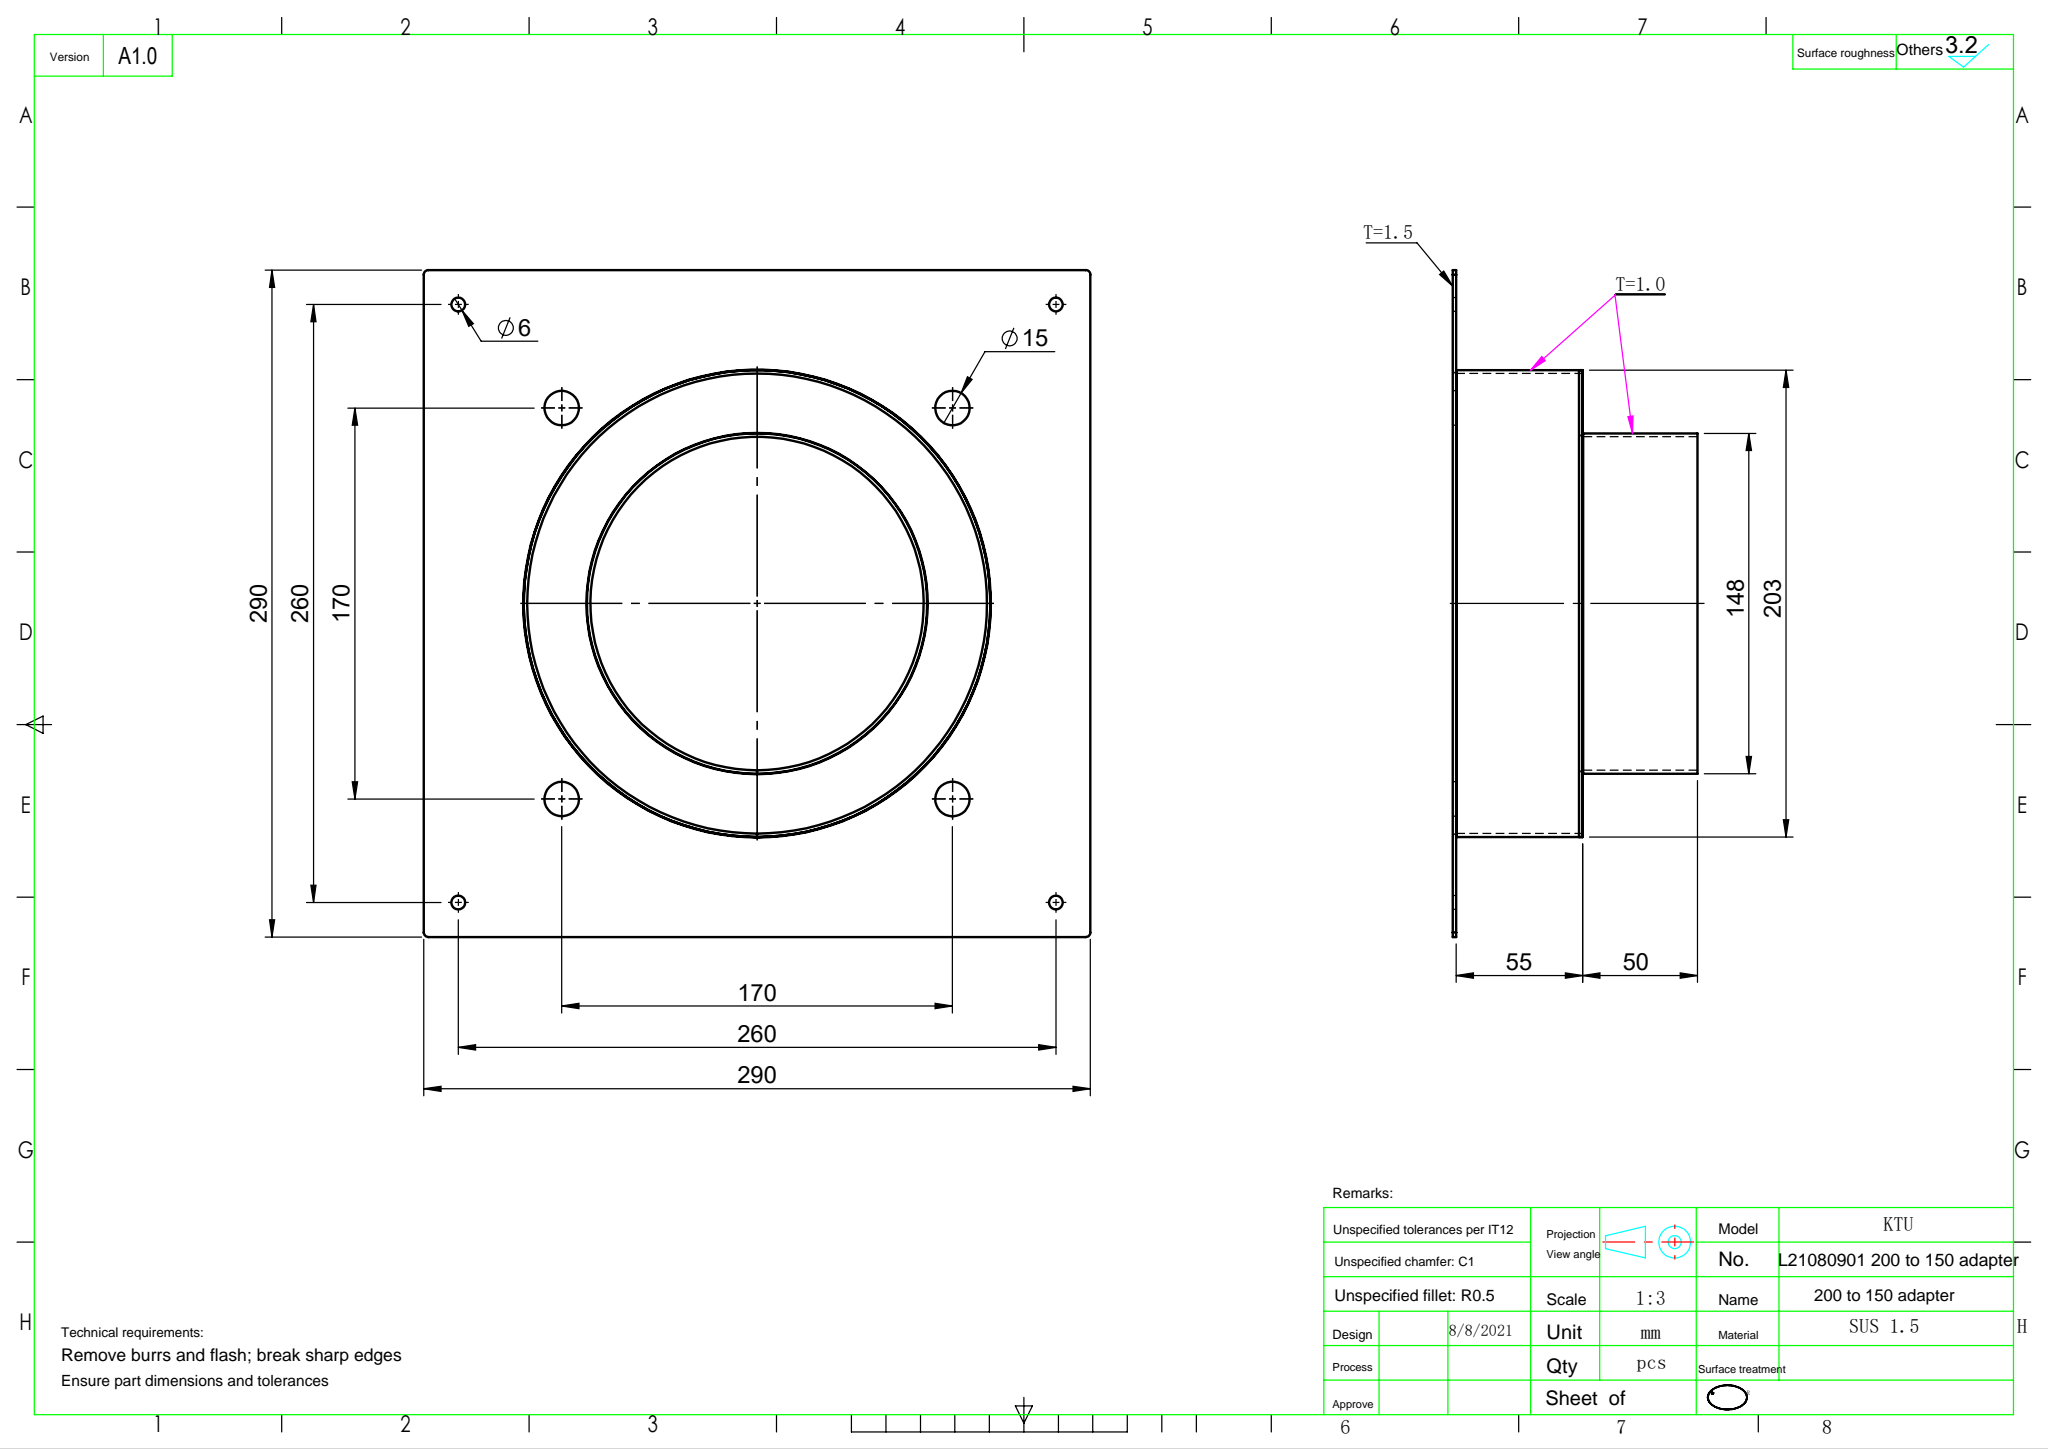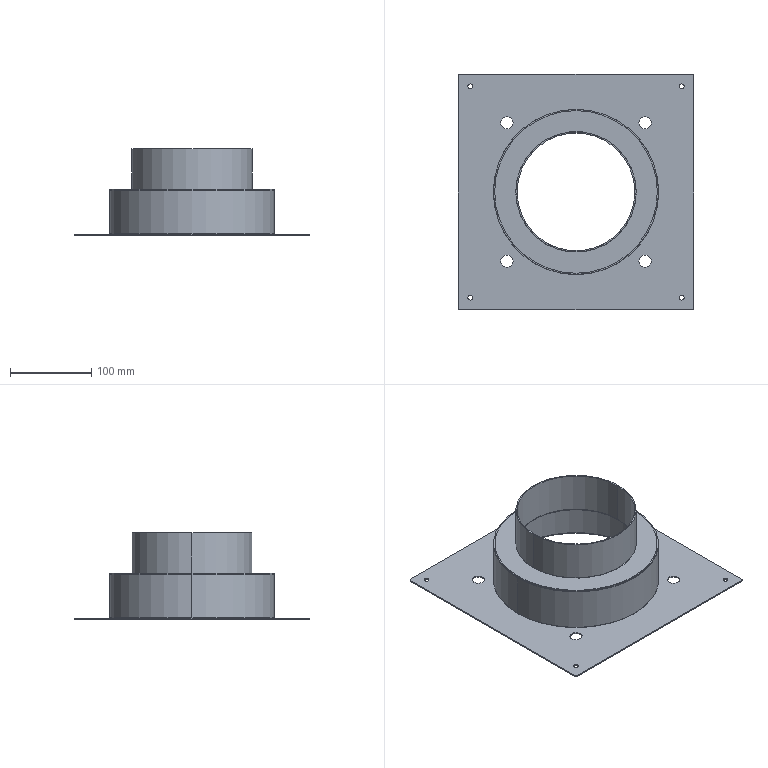Part | SolidWorks | features ICE 3, 3DProfileFeature 2, EdgeFlange 2, FlatPattern 2, SMBaseFlange 2, SheetMetal 2, Fillet 1 | 2 solids | 48 faces | box 290 x 290 x 106.5 mm | volume 187647 mm3 | cylinder 30 | plane 10 | torus 8 | commonest cylinder face diameters 6 x8 15 x8 4 x4 203 x4 145 x2 148 x2